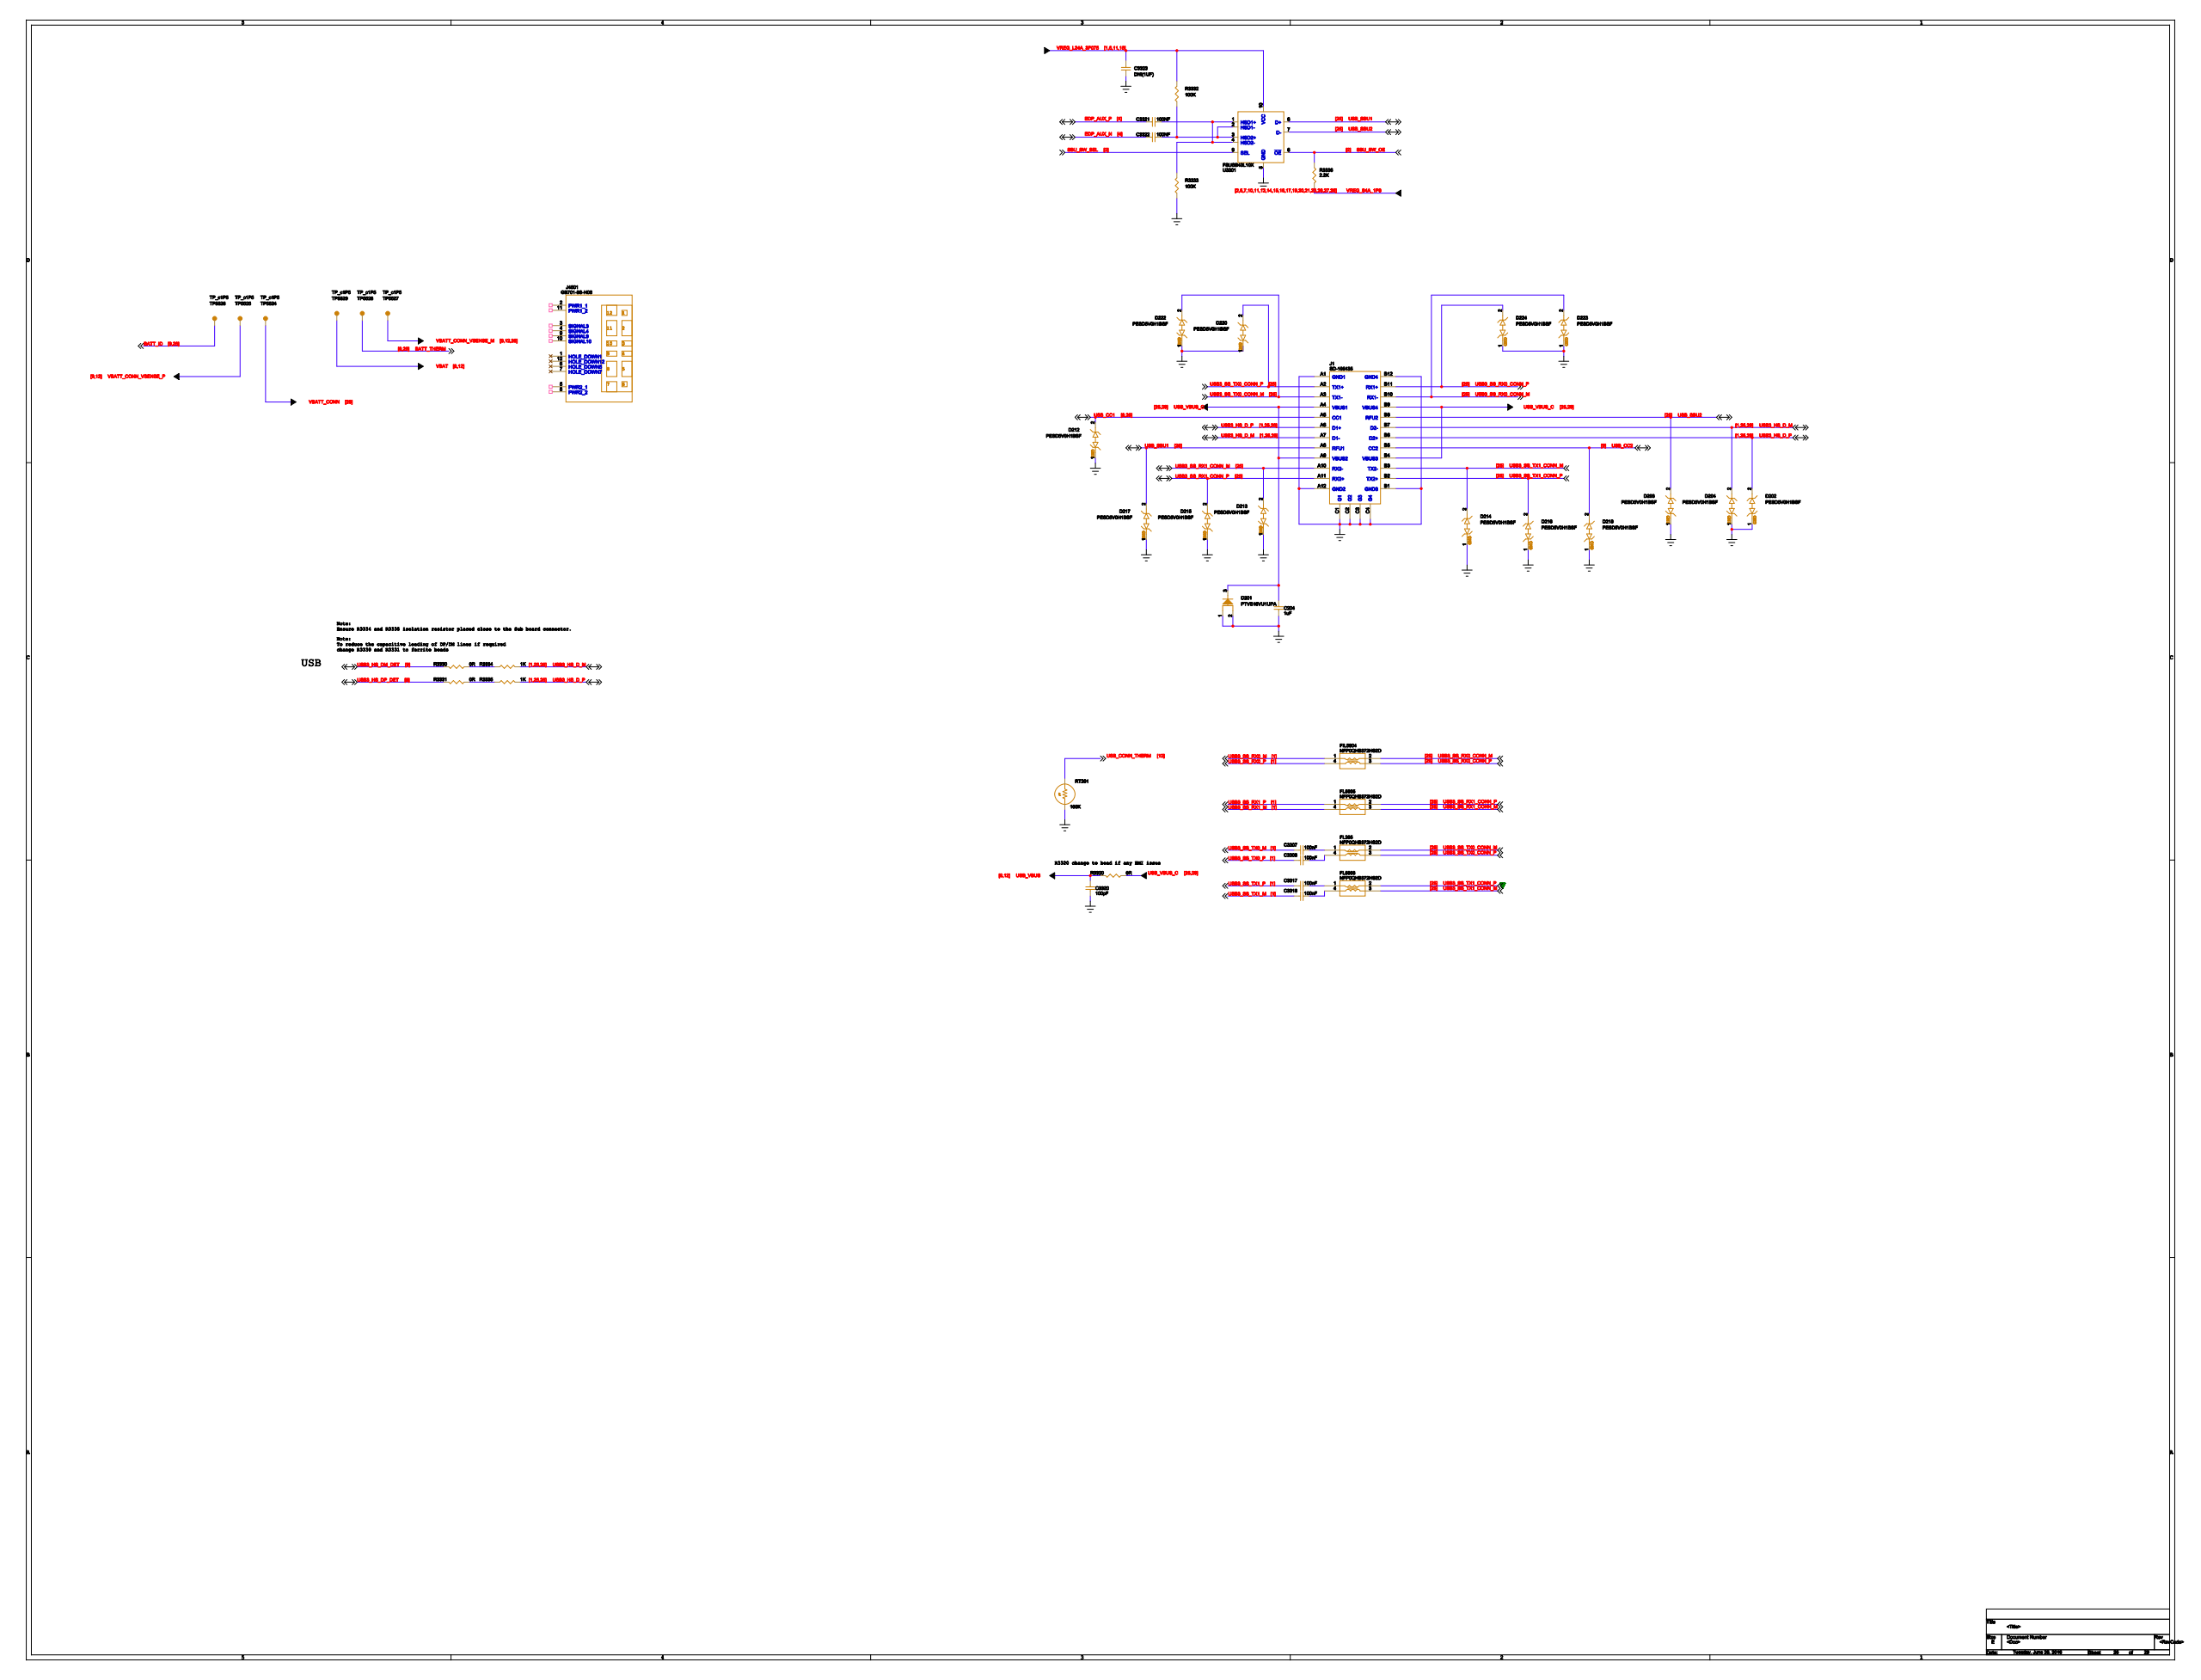Circuit board | Cadence Allegro | 802 parts | 566 nets | one sheet of the schematic
Parts on this sheet (reference | value | footprint):
C204 | 1UF | C0402
C3307 | 100NF | C0201
C3308 | 100NF | C0201
C3317 | 100NF | C0201
C3318 | 100NF | C0201
C3320 | 100pF | C0201
C3321 | 100NF | C0201
C3322 | 100NF | C0201
C3323 | DNI(1UF) | C0402
D201 | PTVS15VU1UPA | DFN2020-3
D202 | PESD5V0H1BSF | DSN0603-2
D203 | PESD5V0H1BSF | DSN0603-2
D204 | PESD5V0H1BSF | DSN0603-2
D212 | PESD5V0H1BSF | DSN0603-2
D213 | PESD5V0H1BSF | DSN0603-2
D214 | PESD5V0H1BSF | DSN0603-2
D215 | PESD5V0H1BSF | DSN0603-2
D216 | PESD5V0H1BSF | DSN0603-2
D217 | PESD5V0H1BSF | DSN0603-2
D218 | PESD5V0H1BSF | DSN0603-2
D220 | PESD5V0H1BSF | DSN0603-2
D222 | PESD5V0H1BSF | DSN0603-2
D223 | PESD5V0H1BSF | DSN0603-2
D224 | PESD5V0H1BSF | DSN0603-2
FIL5804 | NFP0QHB372HS2D | NFP0QHBXXXHS2X
FL205 | NFP0QHB372HS2D | NFP0QHBXXXHS2X
FL5803 | NFP0QHB372HS2D | NFP0QHBXXXHS2X
FL5805 | NFP0QHB372HS2D | NFP0QHBXXXHS2X
J1 | SD-105435 | USB_SD-105435
R3320 | 0R | R0603
R3330 | 0R | R0603
R3331 | 0R | R0603
R3332 | 100K | R0201
R3333 | 100K | R0201
R3334 | 1K | R0201
R3335 | 1K | R0201
R3336 | 2.2K | R0201
RT201 | 100K | R0402
TP5524 | TP_c1P5 | TP_C1P5
TP5525 | TP_c1P5 | TP_C1P5
TP5526 | TP_c1P5 | TP_C1P5
TP5527 | TP_c1P5 | TP_C1P5
TP5528 | TP_c1P5 | TP_C1P5
TP5529 | TP_c1P5 | TP_C1P5
U3301 | FSUSB43L10X | UQFN10_1P6X2P1X0P5_0P65
Nets of these parts (net: part-pin ...):
GND: C204-2 C3320-2 C3323-1 D201-1 D201-2 D202-1 D203-1 D204-1 D212-1 D213-1 D214-1 D215-1 D216-1 D217-1 D218-1 D220-1 D222-1 D223-1 D224-1 R3333-1 RT201-2 U3301-5 J1-A1 J1-A12 J1-B1 J1-B12 J1-C1 J1-C2 J1-C3 J1-C4
VREG_L24A_3P075: C3323-2 R3332-2 U3301-10
VBATT_CONN: TP5524-1
VBATT_CONN_VSENSE_P: TP5525-1
BATT_ID: TP5526-1
VBATT_CONN_VSENSE_M: TP5527-1
BATT_THERM: TP5528-1
VBAT: TP5529-1
USB_VBUS: C3320-1 R3320-2
VREG_S4A_1P8: R3336-2
N441150: C3307-1 FL205-1
USB3_SS_TX0_M: C3307-2
N441262: C3308-1 FL205-4
USB3_SS_TX0_P: C3308-2
N441286: C3317-1 FL5803-1
USB3_SS_TX1_P: C3317-2
N441278: C3318-1 FL5803-4
USB3_SS_TX1_M: C3318-2
EDP_AUX_P: C3321-1
N379686: C3321-2 R3333-2 U3301-1 U3301-4
EDP_AUX_N: C3322-1
N379676: C3322-2 R3332-1 U3301-2 U3301-3
USB3_HS_D_P: D202-2 R3335-2 J1-A6 J1-B6
USB_SBU2: D203-2 U3301-7 J1-B8
USB3_HS_D_M: D204-2 R3334-2 J1-A7 J1-B7
USB_CC1: D212-2 J1-A5
USB3_SS_RX1_CONN_M: D213-2 FL5805-3 J1-A10
USB3_SS_TX1_CONN_M: D214-2 FL5803-3 J1-B3
USB3_SS_RX1_CONN_P: D215-2 FL5805-2 J1-A11
USB3_SS_TX1_CONN_P: D216-2 FL5803-2 J1-B2
USB_SBU1: D217-2 U3301-8 J1-A8
USB_CC2: D218-2 J1-B5
USB3_SS_TX0_CONN_P: D220-2 FL205-3 J1-A2
USB3_SS_TX0_CONN_M: D222-2 FL205-2 J1-A3
USB3_SS_RX0_CONN_M: D223-2 FIL5804-2 J1-B10
USB3_SS_RX0_CONN_P: D224-2 FIL5804-3 J1-B11
USB_VBUS_C: C204-1 D201-3 R3320-1 J1-A4 J1-A9 J1-B4 J1-B9
USB3_SS_RX0_M: FIL5804-1
USB3_SS_RX0_P: FIL5804-4
USB3_SS_RX1_P: FL5805-1
USB3_SS_RX1_M: FL5805-4
SBU_SW_OE: R3336-1 U3301-6
N461913: R3330-1 R3334-1
USB3_HS_DM_DET: R3330-2
N461909: R3331-1 R3335-1
USB3_HS_DP_DET: R3331-2
USB_CONN_THERM: RT201-1
SBU_SW_SEL: U3301-9